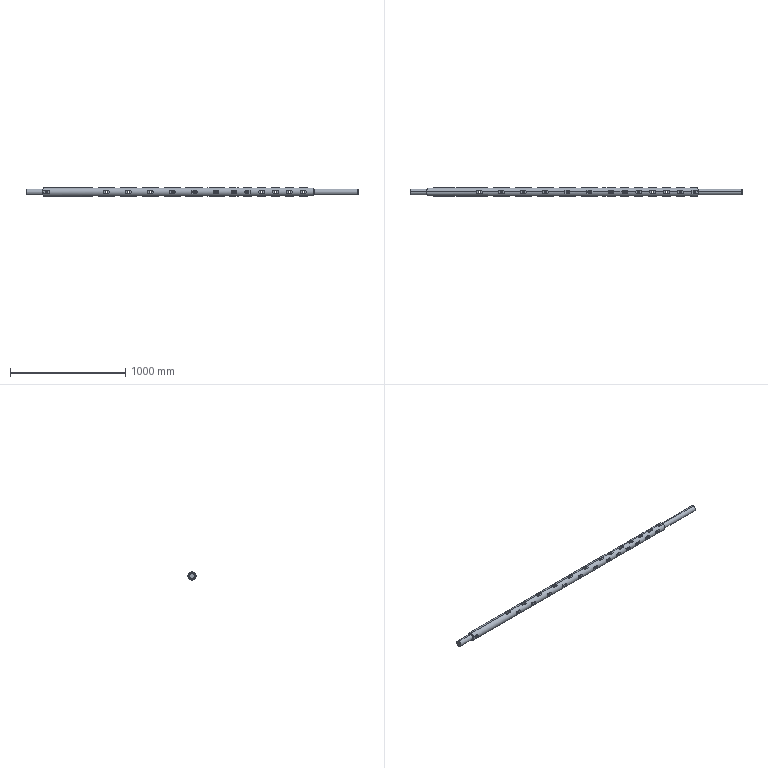Part | SolidWorks | features ICE 18, MirrorPattern 7, LPattern 4, Fillet 2, Chamfer 1, Extrusion 1 | 1 solid | 258 faces | box 2875 x 70 x 70 mm | volume 9321994 mm3 | cylinder 187 | plane 61 | torus 6 | cone 4 | commonest cylinder face diameters 50 x129 20 x52 0.6 x2 14 x2 70 x2